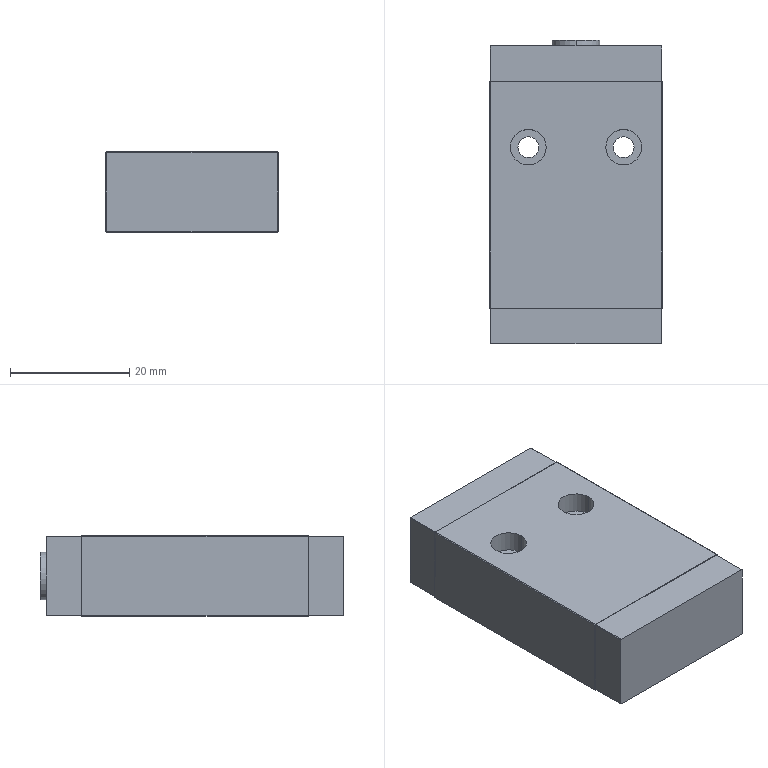Part | SolidWorks | features BaseBody 1 | 1 solid | 50 faces | box 29 x 51 x 13.5 mm | volume 18511 mm3 | plane 34 | cylinder 16 | commonest cylinder face diameters 6 x8 3.5 x4 5 x2 8 x2
STEP:
#1=CARTESIAN_POINT('',(-9.161,10.957,3.5));
#2=VERTEX_POINT('',#1);
#3=CARTESIAN_POINT('',(-15.161,10.957,3.5));
#4=VERTEX_POINT('',#3);
#5=CARTESIAN_POINT('',(-12.161,10.957,3.5));
#6=DIRECTION('',(0.,0.,-1.));
#7=DIRECTION('',(-1.,0.,0.));
#8=AXIS2_PLACEMENT_3D('',#5,#6,#7);
#9=CIRCLE('',#8,3.);
#10=EDGE_CURVE('',#2,#4,#9,.T.);
#11=ORIENTED_EDGE('',*,*,#10,.F.);
#12=CARTESIAN_POINT('',(-9.161,10.957,0.));
#13=VERTEX_POINT('',#12);
#14=CARTESIAN_POINT('',(-9.161,10.957,1.75));
#15=DIRECTION('',(0.,0.,-1.));
#16=VECTOR('',#15,1000.);
#17=LINE('',#14,#16);
#18=EDGE_CURVE('',#2,#13,#17,.T.);
#19=ORIENTED_EDGE('',*,*,#18,.T.);
#20=CARTESIAN_POINT('',(-15.161,10.957,0.));
#21=VERTEX_POINT('',#20);
#22=CARTESIAN_POINT('',(-12.161,10.957,0.));
#23=DIRECTION('',(0.,0.,-1.));
#24=DIRECTION('',(-1.,0.,0.));
#25=AXIS2_PLACEMENT_3D('',#22,#23,#24);
#26=CIRCLE('',#25,3.);
#27=EDGE_CURVE('',#13,#21,#26,.T.);
#28=ORIENTED_EDGE('',*,*,#27,.T.);
#29=CARTESIAN_POINT('',(-15.161,10.957,1.75));
#30=DIRECTION('',(0.,0.,-1.));
#31=VECTOR('',#30,1000.);
#32=LINE('',#29,#31);
#33=EDGE_CURVE('',#4,#21,#32,.T.);
#34=ORIENTED_EDGE('',*,*,#33,.F.);
#35=EDGE_LOOP('',(#11,#19,#28,#34));
#36=FACE_OUTER_BOUND('',#35,.T.);
#37=CARTESIAN_POINT('',(-12.161,10.957,1.75));
#38=DIRECTION('',(0.,0.,-1.));
#39=DIRECTION('',(-1.,0.,0.));
#40=AXIS2_PLACEMENT_3D('',#37,#38,#39);
#41=CYLINDRICAL_SURFACE('',#40,3.);
#42=ADVANCED_FACE('',(#36),#41,.F.);
#43=CARTESIAN_POINT('',(6.839,10.957,3.5));
#44=VERTEX_POINT('',#43);
#45=CARTESIAN_POINT('',(0.8387,10.957,3.5));
#46=VERTEX_POINT('',#45);
#47=CARTESIAN_POINT('',(3.839,10.957,3.5));
#48=DIRECTION('',(0.,0.,-1.));
#49=DIRECTION('',(-1.,0.,0.));
#50=AXIS2_PLACEMENT_3D('',#47,#48,#49);
#51=CIRCLE('',#50,3.);
#52=EDGE_CURVE('',#44,#46,#51,.T.);
#53=ORIENTED_EDGE('',*,*,#52,.F.);
#54=CARTESIAN_POINT('',(6.839,10.957,0.));
#55=VERTEX_POINT('',#54);
#56=CARTESIAN_POINT('',(6.839,10.957,1.75));
#57=DIRECTION('',(0.,0.,-1.));
#58=VECTOR('',#57,1000.);
#59=LINE('',#56,#58);
#60=EDGE_CURVE('',#44,#55,#59,.T.);
#61=ORIENTED_EDGE('',*,*,#60,.T.);
#62=CARTESIAN_POINT('',(0.8387,10.957,0.));
#63=VERTEX_POINT('',#62);
#64=CARTESIAN_POINT('',(3.839,10.957,0.));
#65=DIRECTION('',(0.,0.,-1.));
#66=DIRECTION('',(-1.,0.,0.));
#67=AXIS2_PLACEMENT_3D('',#64,#65,#66);
#68=CIRCLE('',#67,3.);
#69=EDGE_CURVE('',#55,#63,#68,.T.);
#70=ORIENTED_EDGE('',*,*,#69,.T.);
#71=CARTESIAN_POINT('',(0.8387,10.957,1.75));
#72=DIRECTION('',(0.,0.,-1.));
#73=VECTOR('',#72,1000.);
#74=LINE('',#71,#73);
#75=EDGE_CURVE('',#46,#63,#74,.T.);
#76=ORIENTED_EDGE('',*,*,#75,.F.);
#77=EDGE_LOOP('',(#53,#61,#70,#76));
#78=FACE_OUTER_BOUND('',#77,.T.);
#79=CARTESIAN_POINT('',(3.839,10.957,1.75));
#80=DIRECTION('',(0.,0.,-1.));
#81=DIRECTION('',(-1.,0.,0.));
#82=AXIS2_PLACEMENT_3D('',#79,#80,#81);
#83=CYLINDRICAL_SURFACE('',#82,3.);
#84=ADVANCED_FACE('',(#78),#83,.F.);
#85=CARTESIAN_POINT('',(-13.911,10.957,3.5));
#86=VERTEX_POINT('',#85);
#87=CARTESIAN_POINT('',(-10.411,10.957,3.5));
#88=VERTEX_POINT('',#87);
#89=CARTESIAN_POINT('',(-12.161,10.957,3.5));
#90=DIRECTION('',(0.,0.,1.));
#91=DIRECTION('',(1.,0.,0.));
#92=AXIS2_PLACEMENT_3D('',#89,#90,#91);
#93=CIRCLE('',#92,1.75);
#94=EDGE_CURVE('',#86,#88,#93,.T.);
#95=ORIENTED_EDGE('',*,*,#94,.F.);
#96=CARTESIAN_POINT('',(-13.911,10.957,10.));
#97=VERTEX_POINT('',#96);
#98=CARTESIAN_POINT('',(-13.911,10.957,-36.171));
#99=DIRECTION('',(0.,0.,1.));
#100=VECTOR('',#99,1000.);
#101=LINE('',#98,#100);
#102=EDGE_CURVE('',#86,#97,#101,.T.);
#103=ORIENTED_EDGE('',*,*,#102,.T.);
#104=CARTESIAN_POINT('',(-10.411,10.957,10.));
#105=VERTEX_POINT('',#104);
#106=CARTESIAN_POINT('',(-12.161,10.957,10.));
#107=DIRECTION('',(0.,0.,-1.));
#108=DIRECTION('',(1.,0.,0.));
#109=AXIS2_PLACEMENT_3D('',#106,#107,#108);
#110=CIRCLE('',#109,1.75);
#111=EDGE_CURVE('',#105,#97,#110,.T.);
#112=ORIENTED_EDGE('',*,*,#111,.F.);
#113=CARTESIAN_POINT('',(-10.411,10.957,-36.171));
#114=DIRECTION('',(0.,0.,1.));
#115=VECTOR('',#114,1000.);
#116=LINE('',#113,#115);
#117=EDGE_CURVE('',#88,#105,#116,.T.);
#118=ORIENTED_EDGE('',*,*,#117,.F.);
#119=EDGE_LOOP('',(#95,#103,#112,#118));
#120=FACE_OUTER_BOUND('',#119,.T.);
#121=CARTESIAN_POINT('',(-12.161,10.957,-36.171));
#122=DIRECTION('',(0.,0.,1.));
#123=DIRECTION('',(1.,0.,0.));
#124=AXIS2_PLACEMENT_3D('',#121,#122,#123);
#125=CYLINDRICAL_SURFACE('',#124,1.75);
#126=ADVANCED_FACE('',(#120),#125,.F.);
#127=CARTESIAN_POINT('',(2.089,10.957,3.5));
#128=VERTEX_POINT('',#127);
#129=CARTESIAN_POINT('',(5.589,10.957,3.5));
#130=VERTEX_POINT('',#129);
#131=CARTESIAN_POINT('',(3.839,10.957,3.5));
#132=DIRECTION('',(0.,0.,1.));
#133=DIRECTION('',(1.,0.,0.));
#134=AXIS2_PLACEMENT_3D('',#131,#132,#133);
#135=CIRCLE('',#134,1.75);
#136=EDGE_CURVE('',#128,#130,#135,.T.);
#137=ORIENTED_EDGE('',*,*,#136,.F.);
#138=CARTESIAN_POINT('',(2.089,10.957,10.));
#139=VERTEX_POINT('',#138);
#140=CARTESIAN_POINT('',(2.089,10.957,-36.171));
#141=DIRECTION('',(0.,0.,1.));
#142=VECTOR('',#141,1000.);
#143=LINE('',#140,#142);
#144=EDGE_CURVE('',#128,#139,#143,.T.);
#145=ORIENTED_EDGE('',*,*,#144,.T.);
#146=CARTESIAN_POINT('',(5.589,10.957,10.));
#147=VERTEX_POINT('',#146);
#148=CARTESIAN_POINT('',(3.839,10.957,10.));
#149=DIRECTION('',(0.,0.,-1.));
#150=DIRECTION('',(1.,0.,0.));
#151=AXIS2_PLACEMENT_3D('',#148,#149,#150);
#152=CIRCLE('',#151,1.75);
#153=EDGE_CURVE('',#147,#139,#152,.T.);
#154=ORIENTED_EDGE('',*,*,#153,.F.);
#155=CARTESIAN_POINT('',(5.589,10.957,-36.171));
#156=DIRECTION('',(0.,0.,1.));
#157=VECTOR('',#156,1000.);
#158=LINE('',#155,#157);
#159=EDGE_CURVE('',#130,#147,#158,.T.);
#160=ORIENTED_EDGE('',*,*,#159,.F.);
#161=EDGE_LOOP('',(#137,#145,#154,#160));
#162=FACE_OUTER_BOUND('',#161,.T.);
#163=CARTESIAN_POINT('',(3.839,10.957,-36.171));
#164=DIRECTION('',(0.,0.,1.));
#165=DIRECTION('',(1.,0.,0.));
#166=AXIS2_PLACEMENT_3D('',#163,#164,#165);
#167=CYLINDRICAL_SURFACE('',#166,1.75);
#168=ADVANCED_FACE('',(#162),#167,.F.);
#169=CARTESIAN_POINT('',(0.8387,10.957,10.));
#170=VERTEX_POINT('',#169);
#171=CARTESIAN_POINT('',(6.839,10.957,10.));
#172=VERTEX_POINT('',#171);
#173=CARTESIAN_POINT('',(3.839,10.957,10.));
#174=DIRECTION('',(0.,0.,1.));
#175=DIRECTION('',(1.,0.,0.));
#176=AXIS2_PLACEMENT_3D('',#173,#174,#175);
#177=CIRCLE('',#176,3.);
#178=EDGE_CURVE('',#170,#172,#177,.T.);
#179=ORIENTED_EDGE('',*,*,#178,.F.);
#180=CARTESIAN_POINT('',(0.8387,10.957,13.5));
#181=VERTEX_POINT('',#180);
#182=CARTESIAN_POINT('',(0.8387,10.957,11.75));
#183=DIRECTION('',(0.,0.,1.));
#184=VECTOR('',#183,1000.);
#185=LINE('',#182,#184);
#186=EDGE_CURVE('',#170,#181,#185,.T.);
#187=ORIENTED_EDGE('',*,*,#186,.T.);
#188=CARTESIAN_POINT('',(6.839,10.957,13.5));
#189=VERTEX_POINT('',#188);
#190=CARTESIAN_POINT('',(3.839,10.957,13.5));
#191=DIRECTION('',(0.,0.,-1.));
#192=DIRECTION('',(1.,0.,0.));
#193=AXIS2_PLACEMENT_3D('',#190,#191,#192);
#194=CIRCLE('',#193,3.);
#195=EDGE_CURVE('',#189,#181,#194,.T.);
#196=ORIENTED_EDGE('',*,*,#195,.F.);
#197=CARTESIAN_POINT('',(6.839,10.957,11.75));
#198=DIRECTION('',(0.,0.,1.));
#199=VECTOR('',#198,1000.);
#200=LINE('',#197,#199);
#201=EDGE_CURVE('',#172,#189,#200,.T.);
#202=ORIENTED_EDGE('',*,*,#201,.F.);
#203=EDGE_LOOP('',(#179,#187,#196,#202));
#204=FACE_OUTER_BOUND('',#203,.T.);
#205=CARTESIAN_POINT('',(3.839,10.957,11.75));
#206=DIRECTION('',(0.,0.,1.));
#207=DIRECTION('',(1.,0.,0.));
#208=AXIS2_PLACEMENT_3D('',#205,#206,#207);
#209=CYLINDRICAL_SURFACE('',#208,3.);
#210=ADVANCED_FACE('',(#204),#209,.F.);
#211=CARTESIAN_POINT('',(-15.161,10.957,10.));
#212=VERTEX_POINT('',#211);
#213=CARTESIAN_POINT('',(-9.161,10.957,10.));
#214=VERTEX_POINT('',#213);
#215=CARTESIAN_POINT('',(-12.161,10.957,10.));
#216=DIRECTION('',(0.,0.,1.));
#217=DIRECTION('',(1.,0.,0.));
#218=AXIS2_PLACEMENT_3D('',#215,#216,#217);
#219=CIRCLE('',#218,3.);
#220=EDGE_CURVE('',#212,#214,#219,.T.);
#221=ORIENTED_EDGE('',*,*,#220,.F.);
#222=CARTESIAN_POINT('',(-15.161,10.957,13.5));
#223=VERTEX_POINT('',#222);
#224=CARTESIAN_POINT('',(-15.161,10.957,11.75));
#225=DIRECTION('',(0.,0.,1.));
#226=VECTOR('',#225,1000.);
#227=LINE('',#224,#226);
#228=EDGE_CURVE('',#212,#223,#227,.T.);
#229=ORIENTED_EDGE('',*,*,#228,.T.);
#230=CARTESIAN_POINT('',(-9.161,10.957,13.5));
#231=VERTEX_POINT('',#230);
#232=CARTESIAN_POINT('',(-12.161,10.957,13.5));
#233=DIRECTION('',(0.,0.,-1.));
#234=DIRECTION('',(1.,0.,0.));
#235=AXIS2_PLACEMENT_3D('',#232,#233,#234);
#236=CIRCLE('',#235,3.);
#237=EDGE_CURVE('',#231,#223,#236,.T.);
#238=ORIENTED_EDGE('',*,*,#237,.F.);
#239=CARTESIAN_POINT('',(-9.161,10.957,11.75));
#240=DIRECTION('',(0.,0.,1.));
#241=VECTOR('',#240,1000.);
#242=LINE('',#239,#241);
#243=EDGE_CURVE('',#214,#231,#242,.T.);
#244=ORIENTED_EDGE('',*,*,#243,.F.);
#245=EDGE_LOOP('',(#221,#229,#238,#244));
#246=FACE_OUTER_BOUND('',#245,.T.);
#247=CARTESIAN_POINT('',(-12.161,10.957,11.75));
#248=DIRECTION('',(0.,0.,1.));
#249=DIRECTION('',(1.,0.,0.));
#250=AXIS2_PLACEMENT_3D('',#247,#248,#249);
#251=CYLINDRICAL_SURFACE('',#250,3.);
#252=ADVANCED_FACE('',(#246),#251,.F.);
#253=CARTESIAN_POINT('',(-4.161,27.957,2.75));
#254=VERTEX_POINT('',#253);
#255=CARTESIAN_POINT('',(-4.161,27.957,10.75));
#256=VERTEX_POINT('',#255);
#257=CARTESIAN_POINT('',(-4.161,27.957,6.75));
#258=DIRECTION('',(0.,-1.,0.));
#259=DIRECTION('',(0.,0.,1.));
#260=AXIS2_PLACEMENT_3D('',#257,#258,#259);
#261=CIRCLE('',#260,4.);
#262=EDGE_CURVE('',#254,#256,#261,.T.);
#263=ORIENTED_EDGE('',*,*,#262,.F.);
#264=CARTESIAN_POINT('',(-4.161,28.957,2.75));
#265=VERTEX_POINT('',#264);
#266=CARTESIAN_POINT('',(-4.161,27.957,2.75));
#267=DIRECTION('',(0.,1.,0.));
#268=VECTOR('',#267,1000.);
#269=LINE('',#266,#268);
#270=EDGE_CURVE('',#254,#265,#269,.T.);
#271=ORIENTED_EDGE('',*,*,#270,.T.);
#272=CARTESIAN_POINT('',(-4.161,28.957,10.75));
#273=VERTEX_POINT('',#272);
#274=CARTESIAN_POINT('',(-4.161,28.957,6.75));
#275=DIRECTION('',(0.,-1.,0.));
#276=DIRECTION('',(0.,0.,1.));
#277=AXIS2_PLACEMENT_3D('',#274,#275,#276);
#278=CIRCLE('',#277,4.);
#279=EDGE_CURVE('',#265,#273,#278,.T.);
#280=ORIENTED_EDGE('',*,*,#279,.T.);
#281=CARTESIAN_POINT('',(-4.161,27.957,10.75));
#282=DIRECTION('',(0.,1.,0.));
#283=VECTOR('',#282,1000.);
#284=LINE('',#281,#283);
#285=EDGE_CURVE('',#256,#273,#284,.T.);
#286=ORIENTED_EDGE('',*,*,#285,.F.);
#287=EDGE_LOOP('',(#263,#271,#280,#286));
#288=FACE_OUTER_BOUND('',#287,.T.);
#289=CARTESIAN_POINT('',(-4.161,27.957,6.75));
#290=DIRECTION('',(0.,1.,0.));
#291=DIRECTION('',(0.,0.,1.));
#292=AXIS2_PLACEMENT_3D('',#289,#290,#291);
#293=CYLINDRICAL_SURFACE('',#292,4.);
#294=ADVANCED_FACE('',(#288),#293,.T.);
#295=CARTESIAN_POINT('',(-1.661,3.957,6.75));
#296=VERTEX_POINT('',#295);
#297=CARTESIAN_POINT('',(-6.661,3.957,6.75));
#298=VERTEX_POINT('',#297);
#299=CARTESIAN_POINT('',(-4.161,3.957,6.75));
#300=DIRECTION('',(0.,1.,0.));
#301=DIRECTION('',(-1.,0.,0.));
#302=AXIS2_PLACEMENT_3D('',#299,#300,#301);
#303=CIRCLE('',#302,2.5);
#304=EDGE_CURVE('',#296,#298,#303,.T.);
#305=ORIENTED_EDGE('',*,*,#304,.F.);
#306=CARTESIAN_POINT('',(-1.661,28.957,6.75));
#307=VERTEX_POINT('',#306);
#308=CARTESIAN_POINT('',(-1.661,16.457,6.75));
#309=DIRECTION('',(0.,1.,0.));
#310=VECTOR('',#309,1000.);
#311=LINE('',#308,#310);
#312=EDGE_CURVE('',#296,#307,#311,.T.);
#313=ORIENTED_EDGE('',*,*,#312,.T.);
#314=CARTESIAN_POINT('',(-6.661,28.957,6.75));
#315=VERTEX_POINT('',#314);
#316=CARTESIAN_POINT('',(-4.161,28.957,6.75));
#317=DIRECTION('',(0.,1.,0.));
#318=DIRECTION('',(-1.,0.,0.));
#319=AXIS2_PLACEMENT_3D('',#316,#317,#318);
#320=CIRCLE('',#319,2.5);
#321=EDGE_CURVE('',#307,#315,#320,.T.);
#322=ORIENTED_EDGE('',*,*,#321,.T.);
#323=CARTESIAN_POINT('',(-6.661,16.457,6.75));
#324=DIRECTION('',(0.,1.,0.));
#325=VECTOR('',#324,1000.);
#326=LINE('',#323,#325);
#327=EDGE_CURVE('',#298,#315,#326,.T.);
#328=ORIENTED_EDGE('',*,*,#327,.F.);
#329=EDGE_LOOP('',(#305,#313,#322,#328));
#330=FACE_OUTER_BOUND('',#329,.T.);
#331=CARTESIAN_POINT('',(-4.161,16.457,6.75));
#332=DIRECTION('',(0.,1.,0.));
#333=DIRECTION('',(-1.,0.,0.));
#334=AXIS2_PLACEMENT_3D('',#331,#332,#333);
#335=CYLINDRICAL_SURFACE('',#334,2.5);
#336=ADVANCED_FACE('',(#330),#335,.F.);
#337=CARTESIAN_POINT('',(-12.161,10.957,0.));
#338=DIRECTION('',(0.,0.,-1.));
#339=DIRECTION('',(-1.,0.,0.));
#340=AXIS2_PLACEMENT_3D('',#337,#338,#339);
#341=CIRCLE('',#340,3.);
#342=EDGE_CURVE('',#21,#13,#341,.T.);
#343=ORIENTED_EDGE('',*,*,#342,.F.);
#344=ORIENTED_EDGE('',*,*,#27,.F.);
#345=EDGE_LOOP('',(#343,#344));
#346=FACE_BOUND('',#345,.T.);
#347=CARTESIAN_POINT('',(3.839,10.957,0.));
#348=DIRECTION('',(0.,0.,-1.));
#349=DIRECTION('',(-1.,0.,0.));
#350=AXIS2_PLACEMENT_3D('',#347,#348,#349);
#351=CIRCLE('',#350,3.);
#352=EDGE_CURVE('',#63,#55,#351,.T.);
#353=ORIENTED_EDGE('',*,*,#352,.F.);
#354=ORIENTED_EDGE('',*,*,#69,.F.);
#355=EDGE_LOOP('',(#353,#354));
#356=FACE_BOUND('',#355,.T.);
#357=CARTESIAN_POINT('',(10.239,21.957,0.));
#358=VERTEX_POINT('',#357);
#359=CARTESIAN_POINT('',(-18.561,21.957,0.));
#360=VERTEX_POINT('',#359);
#361=CARTESIAN_POINT('',(-4.161,21.957,0.));
#362=DIRECTION('',(-1.,0.,0.));
#363=VECTOR('',#362,1000.);
#364=LINE('',#361,#363);
#365=EDGE_CURVE('',#358,#360,#364,.T.);
#366=ORIENTED_EDGE('',*,*,#365,.F.);
#367=CARTESIAN_POINT('',(10.239,-16.043,0.));
#368=VERTEX_POINT('',#367);
#369=CARTESIAN_POINT('',(10.239,2.957,0.));
#370=DIRECTION('',(0.,1.,0.));
#371=VECTOR('',#370,1000.);
#372=LINE('',#369,#371);
#373=EDGE_CURVE('',#368,#358,#372,.T.);
#374=ORIENTED_EDGE('',*,*,#373,.F.);
#375=CARTESIAN_POINT('',(-18.561,-16.043,0.));
#376=VERTEX_POINT('',#375);
#377=CARTESIAN_POINT('',(-4.161,-16.043,0.));
#378=DIRECTION('',(1.,0.,0.));
#379=VECTOR('',#378,1000.);
#380=LINE('',#377,#379);
#381=EDGE_CURVE('',#376,#368,#380,.T.);
#382=ORIENTED_EDGE('',*,*,#381,.F.);
#383=CARTESIAN_POINT('',(-18.561,2.957,0.));
#384=DIRECTION('',(0.,-1.,0.));
#385=VECTOR('',#384,1000.);
#386=LINE('',#383,#385);
#387=EDGE_CURVE('',#360,#376,#386,.T.);
#388=ORIENTED_EDGE('',*,*,#387,.F.);
#389=EDGE_LOOP('',(#366,#374,#382,#388));
#390=FACE_OUTER_BOUND('',#389,.T.);
#391=CARTESIAN_POINT('',(-4.161,2.957,0.));
#392=DIRECTION('',(0.,0.,1.));
#393=DIRECTION('',(1.,0.,0.));
#394=AXIS2_PLACEMENT_3D('',#391,#392,#393);
#395=PLANE('',#394);
#396=ADVANCED_FACE('',(#346,#356,#390),#395,.F.);
#397=ORIENTED_EDGE('',*,*,#18,.F.);
#398=CARTESIAN_POINT('',(-12.161,10.957,3.5));
#399=DIRECTION('',(0.,0.,-1.));
#400=DIRECTION('',(-1.,0.,0.));
#401=AXIS2_PLACEMENT_3D('',#398,#399,#400);
#402=CIRCLE('',#401,3.);
#403=EDGE_CURVE('',#4,#2,#402,.T.);
#404=ORIENTED_EDGE('',*,*,#403,.F.);
#405=ORIENTED_EDGE('',*,*,#33,.T.);
#406=ORIENTED_EDGE('',*,*,#342,.T.);
#407=EDGE_LOOP('',(#397,#404,#405,#406));
#408=FACE_OUTER_BOUND('',#407,.T.);
#409=CARTESIAN_POINT('',(-12.161,10.957,1.75));
#410=DIRECTION('',(0.,0.,-1.));
#411=DIRECTION('',(-1.,0.,0.));
#412=AXIS2_PLACEMENT_3D('',#409,#410,#411);
#413=CYLINDRICAL_SURFACE('',#412,3.);
#414=ADVANCED_FACE('',(#408),#413,.F.);
#415=ORIENTED_EDGE('',*,*,#60,.F.);
#416=CARTESIAN_POINT('',(3.839,10.957,3.5));
#417=DIRECTION('',(0.,0.,-1.));
#418=DIRECTION('',(-1.,0.,0.));
#419=AXIS2_PLACEMENT_3D('',#416,#417,#418);
#420=CIRCLE('',#419,3.);
#421=EDGE_CURVE('',#46,#44,#420,.T.);
#422=ORIENTED_EDGE('',*,*,#421,.F.);
#423=ORIENTED_EDGE('',*,*,#75,.T.);
#424=ORIENTED_EDGE('',*,*,#352,.T.);
#425=EDGE_LOOP('',(#415,#422,#423,#424));
#426=FACE_OUTER_BOUND('',#425,.T.);
#427=CARTESIAN_POINT('',(3.839,10.957,1.75));
#428=DIRECTION('',(0.,0.,-1.));
#429=DIRECTION('',(-1.,0.,0.));
#430=AXIS2_PLACEMENT_3D('',#427,#428,#429);
#431=CYLINDRICAL_SURFACE('',#430,3.);
#432=ADVANCED_FACE('',(#426),#431,.F.);
#433=CARTESIAN_POINT('',(-18.661,-16.043,0.1));
#434=VERTEX_POINT('',#433);
#435=CARTESIAN_POINT('',(-18.611,-16.043,0.05));
#436=DIRECTION('',(-0.7071,0.,0.7071));
#437=VECTOR('',#436,1000.);
#438=LINE('',#435,#437);
#439=EDGE_CURVE('',#376,#434,#438,.T.);
#440=ORIENTED_EDGE('',*,*,#439,.T.);
#441=CARTESIAN_POINT('',(-18.661,21.957,0.1));
#442=VERTEX_POINT('',#441);
#443=CARTESIAN_POINT('',(-18.661,-6.543,0.1));
#444=DIRECTION('',(0.,1.,0.));
#445=VECTOR('',#444,1000.);
#446=LINE('',#443,#445);
#447=EDGE_CURVE('',#434,#442,#446,.T.);
#448=ORIENTED_EDGE('',*,*,#447,.T.);
#449=CARTESIAN_POINT('',(-18.611,21.957,0.05));
#450=DIRECTION('',(0.7071,0.,-0.7071));
#451=VECTOR('',#450,1000.);
#452=LINE('',#449,#451);
#453=EDGE_CURVE('',#442,#360,#452,.T.);
#454=ORIENTED_EDGE('',*,*,#453,.T.);
#455=ORIENTED_EDGE('',*,*,#387,.T.);
#456=EDGE_LOOP('',(#440,#448,#454,#455));
#457=FACE_OUTER_BOUND('',#456,.T.);
#458=CARTESIAN_POINT('',(-18.611,-6.543,0.05));
#459=DIRECTION('',(-0.7071,0.,-0.7071));
#460=DIRECTION('',(-0.7071,0.,0.7071));
#461=AXIS2_PLACEMENT_3D('',#458,#459,#460);
#462=PLANE('',#461);
#463=ADVANCED_FACE('',(#457),#462,.T.);
#464=CARTESIAN_POINT('',(-18.461,21.957,0.1));
#465=VERTEX_POINT('',#464);
#466=CARTESIAN_POINT('',(10.139,21.957,0.1));
#467=VERTEX_POINT('',#466);
#468=CARTESIAN_POINT('',(-18.661,21.957,0.1));
#469=DIRECTION('',(1.,0.,0.));
#470=VECTOR('',#469,1000.);
#471=LINE('',#468,#470);
#472=EDGE_CURVE('',#465,#467,#471,.T.);
#473=ORIENTED_EDGE('',*,*,#472,.T.);
#474=CARTESIAN_POINT('',(10.239,21.957,0.2));
#475=VERTEX_POINT('',#474);
#476=CARTESIAN_POINT('',(10.189,21.957,0.15));
#477=DIRECTION('',(-0.7071,0.,-0.7071));
#478=VECTOR('',#477,1000.);
#479=LINE('',#476,#478);
#480=EDGE_CURVE('',#475,#467,#479,.T.);
#481=ORIENTED_EDGE('',*,*,#480,.F.);
#482=CARTESIAN_POINT('',(10.239,21.957,13.3));
#483=VERTEX_POINT('',#482);
#484=CARTESIAN_POINT('',(10.239,21.957,0.));
#485=DIRECTION('',(0.,0.,1.));
#486=VECTOR('',#485,1000.);
#487=LINE('',#484,#486);
#488=EDGE_CURVE('',#475,#483,#487,.T.);
#489=ORIENTED_EDGE('',*,*,#488,.T.);
#490=CARTESIAN_POINT('',(10.139,21.957,13.4));
#491=VERTEX_POINT('',#490);
#492=CARTESIAN_POINT('',(10.189,21.957,13.35));
#493=DIRECTION('',(0.7071,0.,-0.7071));
#494=VECTOR('',#493,1000.);
#495=LINE('',#492,#494);
#496=EDGE_CURVE('',#491,#483,#495,.T.);
#497=ORIENTED_EDGE('',*,*,#496,.F.);
#498=CARTESIAN_POINT('',(-18.461,21.957,13.4));
#499=VERTEX_POINT('',#498);
#500=CARTESIAN_POINT('',(-18.661,21.957,13.4));
#501=DIRECTION('',(-1.,0.,0.));
#502=VECTOR('',#501,1000.);
#503=LINE('',#500,#502);
#504=EDGE_CURVE('',#491,#499,#503,.T.);
#505=ORIENTED_EDGE('',*,*,#504,.T.);
#506=CARTESIAN_POINT('',(-18.561,21.957,13.3));
#507=VERTEX_POINT('',#506);
#508=CARTESIAN_POINT('',(-18.511,21.957,13.35));
#509=DIRECTION('',(0.7071,0.,0.7071));
#510=VECTOR('',#509,1000.);
#511=LINE('',#508,#510);
#512=EDGE_CURVE('',#507,#499,#511,.T.);
#513=ORIENTED_EDGE('',*,*,#512,.F.);
#514=CARTESIAN_POINT('',(-18.561,21.957,0.2));
#515=VERTEX_POINT('',#514);
#516=CARTESIAN_POINT('',(-18.561,21.957,0.));
#517=DIRECTION('',(0.,0.,-1.));
#518=VECTOR('',#517,1000.);
#519=LINE('',#516,#518);
#520=EDGE_CURVE('',#507,#515,#519,.T.);
#521=ORIENTED_EDGE('',*,*,#520,.T.);
#522=CARTESIAN_POINT('',(-18.511,21.957,0.15));
#523=DIRECTION('',(-0.7071,0.,0.7071));
#524=VECTOR('',#523,1000.);
#525=LINE('',#522,#524);
#526=EDGE_CURVE('',#465,#515,#525,.T.);
#527=ORIENTED_EDGE('',*,*,#526,.F.);
#528=EDGE_LOOP('',(#473,#481,#489,#497,#505,#513,#521,#527));
#529=FACE_BOUND('',#528,.T.);
#530=CARTESIAN_POINT('',(10.339,21.957,0.1));
#531=VERTEX_POINT('',#530);
#532=CARTESIAN_POINT('',(10.339,21.957,0.1));
#533=DIRECTION('',(-0.7071,0.,-0.7071));
#534=VECTOR('',#533,1000.);
#535=LINE('',#532,#534);
#536=EDGE_CURVE('',#531,#358,#535,.T.);
#537=ORIENTED_EDGE('',*,*,#536,.T.);
#538=ORIENTED_EDGE('',*,*,#365,.T.);
#539=ORIENTED_EDGE('',*,*,#453,.F.);
#540=CARTESIAN_POINT('',(-18.661,21.957,13.4));
#541=VERTEX_POINT('',#540);
#542=CARTESIAN_POINT('',(-18.661,21.957,0.));
#543=DIRECTION('',(0.,0.,1.));
#544=VECTOR('',#543,1000.);
#545=LINE('',#542,#544);
#546=EDGE_CURVE('',#442,#541,#545,.T.);
#547=ORIENTED_EDGE('',*,*,#546,.T.);
#548=CARTESIAN_POINT('',(-18.561,21.957,13.5));
#549=VERTEX_POINT('',#548);
#550=CARTESIAN_POINT('',(-18.611,21.957,13.45));
#551=DIRECTION('',(-0.7071,0.,-0.7071));
#552=VECTOR('',#551,1000.);
#553=LINE('',#550,#552);
#554=EDGE_CURVE('',#549,#541,#553,.T.);
#555=ORIENTED_EDGE('',*,*,#554,.F.);
#556=CARTESIAN_POINT('',(10.239,21.957,13.5));
#557=VERTEX_POINT('',#556);
#558=CARTESIAN_POINT('',(-18.661,21.957,13.5));
#559=DIRECTION('',(1.,0.,0.));
#560=VECTOR('',#559,1000.);
#561=LINE('',#558,#560);
#562=EDGE_CURVE('',#549,#557,#561,.T.);
#563=ORIENTED_EDGE('',*,*,#562,.T.);
#564=CARTESIAN_POINT('',(10.339,21.957,13.4));
#565=VERTEX_POINT('',#564);
#566=CARTESIAN_POINT('',(10.289,21.957,13.45));
#567=DIRECTION('',(-0.7071,0.,0.7071));
#568=VECTOR('',#567,1000.);
#569=LINE('',#566,#568);
#570=EDGE_CURVE('',#565,#557,#569,.T.);
#571=ORIENTED_EDGE('',*,*,#570,.F.);
#572=CARTESIAN_POINT('',(10.339,21.957,0.));
#573=DIRECTION('',(0.,0.,-1.));
#574=VECTOR('',#573,1000.);
#575=LINE('',#572,#574);
#576=EDGE_CURVE('',#565,#531,#575,.T.);
#577=ORIENTED_EDGE('',*,*,#576,.T.);
#578=EDGE_LOOP('',(#537,#538,#539,#547,#555,#563,#571,#577));
#579=FACE_OUTER_BOUND('',#578,.T.);
#580=CARTESIAN_POINT('',(-18.661,21.957,0.));
#581=DIRECTION('',(0.,1.,0.));
#582=DIRECTION('',(0.,0.,1.));
#583=AXIS2_PLACEMENT_3D('',#580,#581,#582);
#584=PLANE('',#583);
#585=ADVANCED_FACE('',(#529,#579),#584,.T.);
#586=ORIENTED_EDGE('',*,*,#536,.F.);
#587=CARTESIAN_POINT('',(10.339,-16.043,0.1));
#588=VERTEX_POINT('',#587);
#589=CARTESIAN_POINT('',(10.339,12.457,0.1));
#590=DIRECTION('',(0.,-1.,0.));
#591=VECTOR('',#590,1000.);
#592=LINE('',#589,#591);
#593=EDGE_CURVE('',#531,#588,#592,.T.);
#594=ORIENTED_EDGE('',*,*,#593,.T.);
#595=CARTESIAN_POINT('',(10.289,-16.043,0.05));
#596=DIRECTION('',(-0.7071,0.,-0.7071));
#597=VECTOR('',#596,1000.);
#598=LINE('',#595,#597);
#599=EDGE_CURVE('',#588,#368,#598,.T.);
#600=ORIENTED_EDGE('',*,*,#599,.T.);
#601=ORIENTED_EDGE('',*,*,#373,.T.);
#602=EDGE_LOOP('',(#586,#594,#600,#601));
#603=FACE_OUTER_BOUND('',#602,.T.);
#604=CARTESIAN_POINT('',(10.289,12.457,0.05));
#605=DIRECTION('',(0.7071,0.,-0.7071));
#606=DIRECTION('',(-0.7071,0.,-0.7071));
#607=AXIS2_PLACEMENT_3D('',#604,#605,#606);
#608=PLANE('',#607);
#609=ADVANCED_FACE('',(#603),#608,.T.);
#610=CARTESIAN_POINT('',(-18.461,-16.043,13.4));
#611=VERTEX_POINT('',#610);
#612=CARTESIAN_POINT('',(10.139,-16.043,13.4));
#613=VERTEX_POINT('',#612);
#614=CARTESIAN_POINT('',(10.339,-16.043,13.4));
#615=DIRECTION('',(1.,0.,0.));
#616=VECTOR('',#615,1000.);
#617=LINE('',#614,#616);
#618=EDGE_CURVE('',#611,#613,#617,.T.);
#619=ORIENTED_EDGE('',*,*,#618,.T.);
#620=CARTESIAN_POINT('',(10.239,-16.043,13.3));
#621=VERTEX_POINT('',#620);
#622=CARTESIAN_POINT('',(10.189,-16.043,13.35));
#623=DIRECTION('',(-0.7071,0.,0.7071));
#624=VECTOR('',#623,1000.);
#625=LINE('',#622,#624);
#626=EDGE_CURVE('',#621,#613,#625,.T.);
#627=ORIENTED_EDGE('',*,*,#626,.F.);
#628=CARTESIAN_POINT('',(10.239,-16.043,0.2));
#629=VERTEX_POINT('',#628);
#630=CARTESIAN_POINT('',(10.239,-16.043,0.));
#631=DIRECTION('',(0.,0.,-1.));
#632=VECTOR('',#631,1000.);
#633=LINE('',#630,#632);
#634=EDGE_CURVE('',#621,#629,#633,.T.);
#635=ORIENTED_EDGE('',*,*,#634,.T.);
#636=CARTESIAN_POINT('',(10.139,-16.043,0.1));
#637=VERTEX_POINT('',#636);
#638=CARTESIAN_POINT('',(10.189,-16.043,0.15));
#639=DIRECTION('',(0.7071,0.,0.7071));
#640=VECTOR('',#639,1000.);
#641=LINE('',#638,#640);
#642=EDGE_CURVE('',#637,#629,#641,.T.);
#643=ORIENTED_EDGE('',*,*,#642,.F.);
#644=CARTESIAN_POINT('',(-18.461,-16.043,0.1));
#645=VERTEX_POINT('',#644);
#646=CARTESIAN_POINT('',(10.339,-16.043,0.1));
#647=DIRECTION('',(-1.,0.,0.));
#648=VECTOR('',#647,1000.);
#649=LINE('',#646,#648);
#650=EDGE_CURVE('',#637,#645,#649,.T.);
#651=ORIENTED_EDGE('',*,*,#650,.T.);
#652=CARTESIAN_POINT('',(-18.561,-16.043,0.2));
#653=VERTEX_POINT('',#652);
#654=CARTESIAN_POINT('',(-18.511,-16.043,0.15));
#655=DIRECTION('',(0.7071,0.,-0.7071));
#656=VECTOR('',#655,1000.);
#657=LINE('',#654,#656);
#658=EDGE_CURVE('',#653,#645,#657,.T.);
#659=ORIENTED_EDGE('',*,*,#658,.F.);
#660=CARTESIAN_POINT('',(-18.561,-16.043,13.3));
#661=VERTEX_POINT('',#660);
#662=CARTESIAN_POINT('',(-18.561,-16.043,0.));
#663=DIRECTION('',(0.,0.,1.));
#664=VECTOR('',#663,1000.);
#665=LINE('',#662,#664);
#666=EDGE_CURVE('',#653,#661,#665,.T.);
#667=ORIENTED_EDGE('',*,*,#666,.T.);
#668=CARTESIAN_POINT('',(-18.511,-16.043,13.35));
#669=DIRECTION('',(-0.7071,0.,-0.7071));
#670=VECTOR('',#669,1000.);
#671=LINE('',#668,#670);
#672=EDGE_CURVE('',#611,#661,#671,.T.);
#673=ORIENTED_EDGE('',*,*,#672,.F.);
#674=EDGE_LOOP('',(#619,#627,#635,#643,#651,#659,#667,#673));
#675=FACE_BOUND('',#674,.T.);
#676=CARTESIAN_POINT('',(-18.661,-16.043,13.4));
#677=VERTEX_POINT('',#676);
#678=CARTESIAN_POINT('',(-18.561,-16.043,13.5));
#679=VERTEX_POINT('',#678);
#680=CARTESIAN_POINT('',(-18.611,-16.043,13.45));
#681=DIRECTION('',(0.7071,0.,0.7071));
#682=VECTOR('',#681,1000.);
#683=LINE('',#680,#682);
#684=EDGE_CURVE('',#677,#679,#683,.T.);
#685=ORIENTED_EDGE('',*,*,#684,.F.);
#686=CARTESIAN_POINT('',(-18.661,-16.043,0.));
#687=DIRECTION('',(0.,0.,-1.));
#688=VECTOR('',#687,1000.);
#689=LINE('',#686,#688);
#690=EDGE_CURVE('',#677,#434,#689,.T.);
#691=ORIENTED_EDGE('',*,*,#690,.T.);
#692=ORIENTED_EDGE('',*,*,#439,.F.);
#693=ORIENTED_EDGE('',*,*,#381,.T.);
#694=ORIENTED_EDGE('',*,*,#599,.F.);
#695=CARTESIAN_POINT('',(10.339,-16.043,13.4));
#696=VERTEX_POINT('',#695);
#697=CARTESIAN_POINT('',(10.339,-16.043,0.));
#698=DIRECTION('',(0.,0.,1.));
#699=VECTOR('',#698,1000.);
#700=LINE('',#697,#699);
#701=EDGE_CURVE('',#588,#696,#700,.T.);
#702=ORIENTED_EDGE('',*,*,#701,.T.);
#703=CARTESIAN_POINT('',(10.239,-16.043,13.5));
#704=VERTEX_POINT('',#703);
#705=CARTESIAN_POINT('',(10.289,-16.043,13.45));
#706=DIRECTION('',(0.7071,0.,-0.7071));
#707=VECTOR('',#706,1000.);
#708=LINE('',#705,#707);
#709=EDGE_CURVE('',#704,#696,#708,.T.);
#710=ORIENTED_EDGE('',*,*,#709,.F.);
#711=CARTESIAN_POINT('',(10.339,-16.043,13.5));
#712=DIRECTION('',(-1.,0.,0.));
#713=VECTOR('',#712,1000.);
#714=LINE('',#711,#713);
#715=EDGE_CURVE('',#704,#679,#714,.T.);
#716=ORIENTED_EDGE('',*,*,#715,.T.);
#717=EDGE_LOOP('',(#685,#691,#692,#693,#694,#702,#710,#716));
#718=FACE_OUTER_BOUND('',#717,.T.);
#719=CARTESIAN_POINT('',(10.339,-16.043,0.));
#720=DIRECTION('',(0.,-1.,0.));
#721=DIRECTION('',(0.,0.,-1.));
#722=AXIS2_PLACEMENT_3D('',#719,#720,#721);
#723=PLANE('',#722);
#724=ADVANCED_FACE('',(#675,#718),#723,.T.);
#725=CARTESIAN_POINT('',(-12.161,10.957,3.5));
#726=DIRECTION('',(0.,0.,1.));
#727=DIRECTION('',(1.,0.,0.));
#728=AXIS2_PLACEMENT_3D('',#725,#726,#727);
#729=CIRCLE('',#728,1.75);
#730=EDGE_CURVE('',#88,#86,#729,.T.);
#731=ORIENTED_EDGE('',*,*,#730,.T.);
#732=ORIENTED_EDGE('',*,*,#94,.T.);
#733=EDGE_LOOP('',(#731,#732));
#734=FACE_BOUND('',#733,.T.);
#735=ORIENTED_EDGE('',*,*,#403,.T.);
#736=ORIENTED_EDGE('',*,*,#10,.T.);
#737=EDGE_LOOP('',(#735,#736));
#738=FACE_OUTER_BOUND('',#737,.T.);
#739=CARTESIAN_POINT('',(-12.161,10.957,3.5));
#740=DIRECTION('',(0.,0.,-1.));
#741=DIRECTION('',(-1.,0.,0.));
#742=AXIS2_PLACEMENT_3D('',#739,#740,#741);
#743=PLANE('',#742);
#744=ADVANCED_FACE('',(#734,#738),#743,.T.);
#745=CARTESIAN_POINT('',(3.839,10.957,3.5));
#746=DIRECTION('',(0.,0.,1.));
#747=DIRECTION('',(1.,0.,0.));
#748=AXIS2_PLACEMENT_3D('',#745,#746,#747);
#749=CIRCLE('',#748,1.75);
#750=EDGE_CURVE('',#130,#128,#749,.T.);
#751=ORIENTED_EDGE('',*,*,#750,.T.);
#752=ORIENTED_EDGE('',*,*,#136,.T.);
#753=EDGE_LOOP('',(#751,#752));
#754=FACE_BOUND('',#753,.T.);
#755=ORIENTED_EDGE('',*,*,#421,.T.);
#756=ORIENTED_EDGE('',*,*,#52,.T.);
#757=EDGE_LOOP('',(#755,#756));
#758=FACE_OUTER_BOUND('',#757,.T.);
#759=CARTESIAN_POINT('',(3.839,10.957,3.5));
#760=DIRECTION('',(0.,0.,-1.));
#761=DIRECTION('',(-1.,0.,0.));
#762=AXIS2_PLACEMENT_3D('',#759,#760,#761);
#763=PLANE('',#762);
#764=ADVANCED_FACE('',(#754,#758),#763,.T.);
#765=CARTESIAN_POINT('',(-18.661,-16.043,13.4));
#766=DIRECTION('',(0.,1.,0.));
#767=VECTOR('',#766,1000.);
#768=LINE('',#765,#767);
#769=EDGE_CURVE('',#677,#541,#768,.T.);
#770=ORIENTED_EDGE('',*,*,#769,.T.);
#771=ORIENTED_EDGE('',*,*,#546,.F.);
#772=ORIENTED_EDGE('',*,*,#447,.F.);
#773=ORIENTED_EDGE('',*,*,#690,.F.);
#774=EDGE_LOOP('',(#770,#771,#772,#773));
#775=FACE_OUTER_BOUND('',#774,.T.);
#776=CARTESIAN_POINT('',(-18.661,-16.043,0.));
#777=DIRECTION('',(-1.,0.,0.));
#778=DIRECTION('',(0.,0.,1.));
#779=AXIS2_PLACEMENT_3D('',#776,#777,#778);
#780=PLANE('',#779);
#781=ADVANCED_FACE('',(#775),#780,.T.);
#782=CARTESIAN_POINT('',(10.139,27.957,0.1));
#783=VERTEX_POINT('',#782);
#784=CARTESIAN_POINT('',(10.139,21.957,0.1));
#785=DIRECTION('',(0.,-1.,0.));
#786=VECTOR('',#785,1000.);
#787=LINE('',#784,#786);
#788=EDGE_CURVE('',#783,#467,#787,.T.);
#789=ORIENTED_EDGE('',*,*,#788,.T.);
#790=ORIENTED_EDGE('',*,*,#472,.F.);
#791=CARTESIAN_POINT('',(-18.461,27.957,0.1));
#792=VERTEX_POINT('',#791);
#793=CARTESIAN_POINT('',(-18.461,21.957,0.1));
#794=DIRECTION('',(0.,1.,0.));
#795=VECTOR('',#794,1000.);
#796=LINE('',#793,#795);
#797=EDGE_CURVE('',#465,#792,#796,.T.);
#798=ORIENTED_EDGE('',*,*,#797,.T.);
#799=CARTESIAN_POINT('',(-18.561,27.957,0.1));
#800=DIRECTION('',(1.,0.,0.));
#801=VECTOR('',#800,1000.);
#802=LINE('',#799,#801);
#803=EDGE_CURVE('',#792,#783,#802,.T.);
#804=ORIENTED_EDGE('',*,*,#803,.T.);
#805=EDGE_LOOP('',(#789,#790,#798,#804));
#806=FACE_OUTER_BOUND('',#805,.T.);
#807=CARTESIAN_POINT('',(-18.561,21.957,0.1));
#808=DIRECTION('',(0.,0.,-1.));
#809=DIRECTION('',(-1.,0.,0.));
#810=AXIS2_PLACEMENT_3D('',#807,#808,#809);
#811=PLANE('',#810);
#812=ADVANCED_FACE('',(#806),#811,.T.);
#813=CARTESIAN_POINT('',(-18.561,27.957,13.3));
#814=VERTEX_POINT('',#813);
#815=CARTESIAN_POINT('',(-18.561,21.957,13.3));
#816=DIRECTION('',(0.,1.,0.));
#817=VECTOR('',#816,1000.);
#818=LINE('',#815,#817);
#819=EDGE_CURVE('',#507,#814,#818,.T.);
#820=ORIENTED_EDGE('',*,*,#819,.T.);
#821=CARTESIAN_POINT('',(-18.561,27.957,0.2));
#822=VERTEX_POINT('',#821);
#823=CARTESIAN_POINT('',(-18.561,27.957,13.4));
#824=DIRECTION('',(0.,0.,-1.));
#825=VECTOR('',#824,1000.);
#826=LINE('',#823,#825);
#827=EDGE_CURVE('',#814,#822,#826,.T.);
#828=ORIENTED_EDGE('',*,*,#827,.T.);
#829=CARTESIAN_POINT('',(-18.561,21.957,0.2));
#830=DIRECTION('',(0.,-1.,0.));
#831=VECTOR('',#830,1000.);
#832=LINE('',#829,#831);
#833=EDGE_CURVE('',#822,#515,#832,.T.);
#834=ORIENTED_EDGE('',*,*,#833,.T.);
#835=ORIENTED_EDGE('',*,*,#520,.F.);
#836=EDGE_LOOP('',(#820,#828,#834,#835));
#837=FACE_OUTER_BOUND('',#836,.T.);
#838=CARTESIAN_POINT('',(-18.561,21.957,13.4));
#839=DIRECTION('',(-1.,0.,0.));
#840=DIRECTION('',(0.,0.,1.));
#841=AXIS2_PLACEMENT_3D('',#838,#839,#840);
#842=PLANE('',#841);
#843=ADVANCED_FACE('',(#837),#842,.T.);
#844=CARTESIAN_POINT('',(10.139,27.957,13.4));
#845=VERTEX_POINT('',#844);
#846=CARTESIAN_POINT('',(10.139,21.957,13.4));
#847=DIRECTION('',(0.,1.,0.));
#848=VECTOR('',#847,1000.);
#849=LINE('',#846,#848);
#850=EDGE_CURVE('',#491,#845,#849,.T.);
#851=ORIENTED_EDGE('',*,*,#850,.T.);
#852=CARTESIAN_POINT('',(-18.461,27.957,13.4));
#853=VERTEX_POINT('',#852);
#854=CARTESIAN_POINT('',(10.239,27.957,13.4));
#855=DIRECTION('',(-1.,0.,0.));
#856=VECTOR('',#855,1000.);
#857=LINE('',#854,#856);
#858=EDGE_CURVE('',#845,#853,#857,.T.);
#859=ORIENTED_EDGE('',*,*,#858,.T.);
#860=CARTESIAN_POINT('',(-18.461,21.957,13.4));
#861=DIRECTION('',(0.,-1.,0.));
#862=VECTOR('',#861,1000.);
#863=LINE('',#860,#862);
#864=EDGE_CURVE('',#853,#499,#863,.T.);
#865=ORIENTED_EDGE('',*,*,#864,.T.);
#866=ORIENTED_EDGE('',*,*,#504,.F.);
#867=EDGE_LOOP('',(#851,#859,#865,#866));
#868=FACE_OUTER_BOUND('',#867,.T.);
#869=CARTESIAN_POINT('',(10.239,21.957,13.4));
#870=DIRECTION('',(0.,0.,1.));
#871=DIRECTION('',(1.,0.,0.));
#872=AXIS2_PLACEMENT_3D('',#869,#870,#871);
#873=PLANE('',#872);
#874=ADVANCED_FACE('',(#868),#873,.T.);
#875=CARTESIAN_POINT('',(10.239,27.957,13.3));
#876=VERTEX_POINT('',#875);
#877=CARTESIAN_POINT('',(10.239,21.957,13.3));
#878=DIRECTION('',(0.,-1.,0.));
#879=VECTOR('',#878,1000.);
#880=LINE('',#877,#879);
#881=EDGE_CURVE('',#876,#483,#880,.T.);
#882=ORIENTED_EDGE('',*,*,#881,.T.);
#883=ORIENTED_EDGE('',*,*,#488,.F.);
#884=CARTESIAN_POINT('',(10.239,27.957,0.2));
#885=VERTEX_POINT('',#884);
#886=CARTESIAN_POINT('',(10.239,21.957,0.2));
#887=DIRECTION('',(0.,1.,0.));
#888=VECTOR('',#887,1000.);
#889=LINE('',#886,#888);
#890=EDGE_CURVE('',#475,#885,#889,.T.);
#891=ORIENTED_EDGE('',*,*,#890,.T.);
#892=CARTESIAN_POINT('',(10.239,27.957,0.1));
#893=DIRECTION('',(0.,0.,1.));
#894=VECTOR('',#893,1000.);
#895=LINE('',#892,#894);
#896=EDGE_CURVE('',#885,#876,#895,.T.);
#897=ORIENTED_EDGE('',*,*,#896,.T.);
#898=EDGE_LOOP('',(#882,#883,#891,#897));
#899=FACE_OUTER_BOUND('',#898,.T.);
#900=CARTESIAN_POINT('',(10.239,21.957,0.1));
#901=DIRECTION('',(1.,0.,0.));
#902=DIRECTION('',(0.,0.,-1.));
#903=AXIS2_PLACEMENT_3D('',#900,#901,#902);
#904=PLANE('',#903);
#905=ADVANCED_FACE('',(#899),#904,.T.);
#906=CARTESIAN_POINT('',(10.339,21.957,13.4));
#907=DIRECTION('',(0.,-1.,0.));
#908=VECTOR('',#907,1000.);
#909=LINE('',#906,#908);
#910=EDGE_CURVE('',#565,#696,#909,.T.);
#911=ORIENTED_EDGE('',*,*,#910,.T.);
#912=ORIENTED_EDGE('',*,*,#701,.F.);
#913=ORIENTED_EDGE('',*,*,#593,.F.);
#914=ORIENTED_EDGE('',*,*,#576,.F.);
#915=EDGE_LOOP('',(#911,#912,#913,#914));
#916=FACE_OUTER_BOUND('',#915,.T.);
#917=CARTESIAN_POINT('',(10.339,21.957,0.));
#918=DIRECTION('',(1.,0.,0.));
#919=DIRECTION('',(0.,0.,-1.));
#920=AXIS2_PLACEMENT_3D('',#917,#918,#919);
#921=PLANE('',#920);
#922=ADVANCED_FACE('',(#916),#921,.T.);
#923=ORIENTED_EDGE('',*,*,#195,.T.);
#924=CARTESIAN_POINT('',(3.839,10.957,13.5));
#925=DIRECTION('',(0.,0.,-1.));
#926=DIRECTION('',(1.,0.,0.));
#927=AXIS2_PLACEMENT_3D('',#924,#925,#926);
#928=CIRCLE('',#927,3.);
#929=EDGE_CURVE('',#181,#189,#928,.T.);
#930=ORIENTED_EDGE('',*,*,#929,.T.);
#931=EDGE_LOOP('',(#923,#930));
#932=FACE_BOUND('',#931,.T.);
#933=ORIENTED_EDGE('',*,*,#237,.T.);
#934=CARTESIAN_POINT('',(-12.161,10.957,13.5));
#935=DIRECTION('',(0.,0.,-1.));
#936=DIRECTION('',(1.,0.,0.));
#937=AXIS2_PLACEMENT_3D('',#934,#935,#936);
#938=CIRCLE('',#937,3.);
#939=EDGE_CURVE('',#223,#231,#938,.T.);
#940=ORIENTED_EDGE('',*,*,#939,.T.);
#941=EDGE_LOOP('',(#933,#940));
#942=FACE_BOUND('',#941,.T.);
#943=CARTESIAN_POINT('',(10.239,2.957,13.5));
#944=DIRECTION('',(0.,1.,0.));
#945=VECTOR('',#944,1000.);
#946=LINE('',#943,#945);
#947=EDGE_CURVE('',#704,#557,#946,.T.);
#948=ORIENTED_EDGE('',*,*,#947,.T.);
#949=ORIENTED_EDGE('',*,*,#562,.F.);
#950=CARTESIAN_POINT('',(-18.561,2.957,13.5));
#951=DIRECTION('',(0.,-1.,0.));
#952=VECTOR('',#951,1000.);
#953=LINE('',#950,#952);
#954=EDGE_CURVE('',#549,#679,#953,.T.);
#955=ORIENTED_EDGE('',*,*,#954,.T.);
#956=ORIENTED_EDGE('',*,*,#715,.F.);
#957=EDGE_LOOP('',(#948,#949,#955,#956));
#958=FACE_OUTER_BOUND('',#957,.T.);
#959=CARTESIAN_POINT('',(-4.161,2.957,13.5));
#960=DIRECTION('',(0.,0.,1.));
#961=DIRECTION('',(1.,0.,0.));
#962=AXIS2_PLACEMENT_3D('',#959,#960,#961);
#963=PLANE('',#962);
#964=ADVANCED_FACE('',(#932,#942,#958),#963,.T.);
#965=CARTESIAN_POINT('',(10.139,-22.043,13.4));
#966=VERTEX_POINT('',#965);
#967=CARTESIAN_POINT('',(10.139,-16.043,13.4));
#968=DIRECTION('',(0.,1.,0.));
#969=VECTOR('',#968,1000.);
#970=LINE('',#967,#969);
#971=EDGE_CURVE('',#966,#613,#970,.T.);
#972=ORIENTED_EDGE('',*,*,#971,.T.);
#973=ORIENTED_EDGE('',*,*,#618,.F.);
#974=CARTESIAN_POINT('',(-18.461,-22.043,13.4));
#975=VERTEX_POINT('',#974);
#976=CARTESIAN_POINT('',(-18.461,-16.043,13.4));
#977=DIRECTION('',(0.,-1.,0.));
#978=VECTOR('',#977,1000.);
#979=LINE('',#976,#978);
#980=EDGE_CURVE('',#611,#975,#979,.T.);
#981=ORIENTED_EDGE('',*,*,#980,.T.);
#982=CARTESIAN_POINT('',(-18.561,-22.043,13.4));
#983=DIRECTION('',(1.,0.,0.));
#984=VECTOR('',#983,1000.);
#985=LINE('',#982,#984);
#986=EDGE_CURVE('',#975,#966,#985,.T.);
#987=ORIENTED_EDGE('',*,*,#986,.T.);
#988=EDGE_LOOP('',(#972,#973,#981,#987));
#989=FACE_OUTER_BOUND('',#988,.T.);
#990=CARTESIAN_POINT('',(-18.561,-16.043,13.4));
#991=DIRECTION('',(0.,0.,1.));
#992=DIRECTION('',(1.,0.,0.));
#993=AXIS2_PLACEMENT_3D('',#990,#991,#992);
#994=PLANE('',#993);
#995=ADVANCED_FACE('',(#989),#994,.T.);
#996=CARTESIAN_POINT('',(-18.561,-22.043,13.3));
#997=VERTEX_POINT('',#996);
#998=CARTESIAN_POINT('',(-18.561,-16.043,13.3));
#999=DIRECTION('',(0.,1.,0.));
#1000=VECTOR('',#999,1000.);
#1001=LINE('',#998,#1000);
#1002=EDGE_CURVE('',#997,#661,#1001,.T.);
#1003=ORIENTED_EDGE('',*,*,#1002,.T.);
#1004=ORIENTED_EDGE('',*,*,#666,.F.);
#1005=CARTESIAN_POINT('',(-18.561,-22.043,0.2));
#1006=VERTEX_POINT('',#1005);
#1007=CARTESIAN_POINT('',(-18.561,-16.043,0.2));
#1008=DIRECTION('',(0.,-1.,0.));
#1009=VECTOR('',#1008,1000.);
#1010=LINE('',#1007,#1009);
#1011=EDGE_CURVE('',#653,#1006,#1010,.T.);
#1012=ORIENTED_EDGE('',*,*,#1011,.T.);
#1013=CARTESIAN_POINT('',(-18.561,-22.043,0.1));
#1014=DIRECTION('',(0.,0.,1.));
#1015=VECTOR('',#1014,1000.);
#1016=LINE('',#1013,#1015);
#1017=EDGE_CURVE('',#1006,#997,#1016,.T.);
#1018=ORIENTED_EDGE('',*,*,#1017,.T.);
#1019=EDGE_LOOP('',(#1003,#1004,#1012,#1018));
#1020=FACE_OUTER_BOUND('',#1019,.T.);
#1021=CARTESIAN_POINT('',(-18.561,-16.043,0.1));
#1022=DIRECTION('',(-1.,0.,0.));
#1023=DIRECTION('',(0.,0.,1.));
#1024=AXIS2_PLACEMENT_3D('',#1021,#1022,#1023);
#1025=PLANE('',#1024);
#1026=ADVANCED_FACE('',(#1020),#1025,.T.);
#1027=CARTESIAN_POINT('',(10.139,-22.043,0.1));
#1028=VERTEX_POINT('',#1027);
#1029=CARTESIAN_POINT('',(10.139,-16.043,0.1));
#1030=DIRECTION('',(0.,-1.,0.));
#1031=VECTOR('',#1030,1000.);
#1032=LINE('',#1029,#1031);
#1033=EDGE_CURVE('',#637,#1028,#1032,.T.);
#1034=ORIENTED_EDGE('',*,*,#1033,.T.);
#1035=CARTESIAN_POINT('',(-18.461,-22.043,0.1));
#1036=VERTEX_POINT('',#1035);
#1037=CARTESIAN_POINT('',(10.239,-22.043,0.1));
#1038=DIRECTION('',(-1.,0.,0.));
#1039=VECTOR('',#1038,1000.);
#1040=LINE('',#1037,#1039);
#1041=EDGE_CURVE('',#1028,#1036,#1040,.T.);
#1042=ORIENTED_EDGE('',*,*,#1041,.T.);
#1043=CARTESIAN_POINT('',(-18.461,-16.043,0.1));
#1044=DIRECTION('',(0.,1.,0.));
#1045=VECTOR('',#1044,1000.);
#1046=LINE('',#1043,#1045);
#1047=EDGE_CURVE('',#1036,#645,#1046,.T.);
#1048=ORIENTED_EDGE('',*,*,#1047,.T.);
#1049=ORIENTED_EDGE('',*,*,#650,.F.);
#1050=EDGE_LOOP('',(#1034,#1042,#1048,#1049));
#1051=FACE_OUTER_BOUND('',#1050,.T.);
#1052=CARTESIAN_POINT('',(10.239,-16.043,0.1));
#1053=DIRECTION('',(0.,0.,-1.));
#1054=DIRECTION('',(-1.,0.,0.));
#1055=AXIS2_PLACEMENT_3D('',#1052,#1053,#1054);
#1056=PLANE('',#1055);
#1057=ADVANCED_FACE('',(#1051),#1056,.T.);
#1058=CARTESIAN_POINT('',(10.239,-22.043,13.3));
#1059=VERTEX_POINT('',#1058);
#1060=CARTESIAN_POINT('',(10.239,-16.043,13.3));
#1061=DIRECTION('',(0.,-1.,0.));
#1062=VECTOR('',#1061,1000.);
#1063=LINE('',#1060,#1062);
#1064=EDGE_CURVE('',#621,#1059,#1063,.T.);
#1065=ORIENTED_EDGE('',*,*,#1064,.T.);
#1066=CARTESIAN_POINT('',(10.239,-22.043,0.2));
#1067=VERTEX_POINT('',#1066);
#1068=CARTESIAN_POINT('',(10.239,-22.043,13.4));
#1069=DIRECTION('',(0.,0.,-1.));
#1070=VECTOR('',#1069,1000.);
#1071=LINE('',#1068,#1070);
#1072=EDGE_CURVE('',#1059,#1067,#1071,.T.);
#1073=ORIENTED_EDGE('',*,*,#1072,.T.);
#1074=CARTESIAN_POINT('',(10.239,-16.043,0.2));
#1075=DIRECTION('',(0.,1.,0.));
#1076=VECTOR('',#1075,1000.);
#1077=LINE('',#1074,#1076);
#1078=EDGE_CURVE('',#1067,#629,#1077,.T.);
#1079=ORIENTED_EDGE('',*,*,#1078,.T.);
#1080=ORIENTED_EDGE('',*,*,#634,.F.);
#1081=EDGE_LOOP('',(#1065,#1073,#1079,#1080));
#1082=FACE_OUTER_BOUND('',#1081,.T.);
#1083=CARTESIAN_POINT('',(10.239,-16.043,13.4));
#1084=DIRECTION('',(1.,0.,0.));
#1085=DIRECTION('',(0.,0.,-1.));
#1086=AXIS2_PLACEMENT_3D('',#1083,#1084,#1085);
#1087=PLANE('',#1086);
#1088=ADVANCED_FACE('',(#1082),#1087,.T.);
#1089=ORIENTED_EDGE('',*,*,#102,.F.);
#1090=ORIENTED_EDGE('',*,*,#730,.F.);
#1091=ORIENTED_EDGE('',*,*,#117,.T.);
#1092=CARTESIAN_POINT('',(-12.161,10.957,10.));
#1093=DIRECTION('',(0.,0.,-1.));
#1094=DIRECTION('',(1.,0.,0.));
#1095=AXIS2_PLACEMENT_3D('',#1092,#1093,#1094);
#1096=CIRCLE('',#1095,1.75);
#1097=EDGE_CURVE('',#97,#105,#1096,.T.);
#1098=ORIENTED_EDGE('',*,*,#1097,.F.);
#1099=EDGE_LOOP('',(#1089,#1090,#1091,#1098));
#1100=FACE_OUTER_BOUND('',#1099,.T.);
#1101=CARTESIAN_POINT('',(-12.161,10.957,-36.171));
#1102=DIRECTION('',(0.,0.,1.));
#1103=DIRECTION('',(1.,0.,0.));
#1104=AXIS2_PLACEMENT_3D('',#1101,#1102,#1103);
#1105=CYLINDRICAL_SURFACE('',#1104,1.75);
#1106=ADVANCED_FACE('',(#1100),#1105,.F.);
#1107=ORIENTED_EDGE('',*,*,#144,.F.);
#1108=ORIENTED_EDGE('',*,*,#750,.F.);
#1109=ORIENTED_EDGE('',*,*,#159,.T.);
#1110=CARTESIAN_POINT('',(3.839,10.957,10.));
#1111=DIRECTION('',(0.,0.,-1.));
#1112=DIRECTION('',(1.,0.,0.));
#1113=AXIS2_PLACEMENT_3D('',#1110,#1111,#1112);
#1114=CIRCLE('',#1113,1.75);
#1115=EDGE_CURVE('',#139,#147,#1114,.T.);
#1116=ORIENTED_EDGE('',*,*,#1115,.F.);
#1117=EDGE_LOOP('',(#1107,#1108,#1109,#1116));
#1118=FACE_OUTER_BOUND('',#1117,.T.);
#1119=CARTESIAN_POINT('',(3.839,10.957,-36.171));
#1120=DIRECTION('',(0.,0.,1.));
#1121=DIRECTION('',(1.,0.,0.));
#1122=AXIS2_PLACEMENT_3D('',#1119,#1120,#1121);
#1123=CYLINDRICAL_SURFACE('',#1122,1.75);
#1124=ADVANCED_FACE('',(#1118),#1123,.F.);
#1125=ORIENTED_EDGE('',*,*,#684,.T.);
#1126=ORIENTED_EDGE('',*,*,#954,.F.);
#1127=ORIENTED_EDGE('',*,*,#554,.T.);
#1128=ORIENTED_EDGE('',*,*,#769,.F.);
#1129=EDGE_LOOP('',(#1125,#1126,#1127,#1128));
#1130=FACE_OUTER_BOUND('',#1129,.T.);
#1131=CARTESIAN_POINT('',(-18.611,-6.543,13.45));
#1132=DIRECTION('',(-0.7071,0.,0.7071));
#1133=DIRECTION('',(0.7071,0.,0.7071));
#1134=AXIS2_PLACEMENT_3D('',#1131,#1132,#1133);
#1135=PLANE('',#1134);
#1136=ADVANCED_FACE('',(#1130),#1135,.T.);
#1137=ORIENTED_EDGE('',*,*,#480,.T.);
#1138=ORIENTED_EDGE('',*,*,#788,.F.);
#1139=CARTESIAN_POINT('',(10.189,27.957,0.15));
#1140=DIRECTION('',(0.7071,0.,0.7071));
#1141=VECTOR('',#1140,1000.);
#1142=LINE('',#1139,#1141);
#1143=EDGE_CURVE('',#783,#885,#1142,.T.);
#1144=ORIENTED_EDGE('',*,*,#1143,.T.);
#1145=ORIENTED_EDGE('',*,*,#890,.F.);
#1146=EDGE_LOOP('',(#1137,#1138,#1144,#1145));
#1147=FACE_OUTER_BOUND('',#1146,.T.);
#1148=CARTESIAN_POINT('',(10.189,21.957,0.15));
#1149=DIRECTION('',(0.7071,0.,-0.7071));
#1150=DIRECTION('',(-0.7071,0.,-0.7071));
#1151=AXIS2_PLACEMENT_3D('',#1148,#1149,#1150);
#1152=PLANE('',#1151);
#1153=ADVANCED_FACE('',(#1147),#1152,.T.);
#1154=CARTESIAN_POINT('',(-4.161,27.957,6.75));
#1155=DIRECTION('',(0.,-1.,0.));
#1156=DIRECTION('',(0.,0.,1.));
#1157=AXIS2_PLACEMENT_3D('',#1154,#1155,#1156);
#1158=CIRCLE('',#1157,4.);
#1159=EDGE_CURVE('',#256,#254,#1158,.T.);
#1160=ORIENTED_EDGE('',*,*,#1159,.T.);
#1161=ORIENTED_EDGE('',*,*,#262,.T.);
#1162=EDGE_LOOP('',(#1160,#1161));
#1163=FACE_BOUND('',#1162,.T.);
#1164=ORIENTED_EDGE('',*,*,#1143,.F.);
#1165=ORIENTED_EDGE('',*,*,#803,.F.);
#1166=CARTESIAN_POINT('',(-18.461,27.957,0.1));
#1167=DIRECTION('',(-0.7071,0.,0.7071));
#1168=VECTOR('',#1167,1000.);
#1169=LINE('',#1166,#1168);
#1170=EDGE_CURVE('',#792,#822,#1169,.T.);
#1171=ORIENTED_EDGE('',*,*,#1170,.T.);
#1172=ORIENTED_EDGE('',*,*,#827,.F.);
#1173=CARTESIAN_POINT('',(-18.561,27.957,13.3));
#1174=DIRECTION('',(0.7071,0.,0.7071));
#1175=VECTOR('',#1174,1000.);
#1176=LINE('',#1173,#1175);
#1177=EDGE_CURVE('',#814,#853,#1176,.T.);
#1178=ORIENTED_EDGE('',*,*,#1177,.T.);
#1179=ORIENTED_EDGE('',*,*,#858,.F.);
#1180=CARTESIAN_POINT('',(10.139,27.957,13.4));
#1181=DIRECTION('',(0.7071,0.,-0.7071));
#1182=VECTOR('',#1181,1000.);
#1183=LINE('',#1180,#1182);
#1184=EDGE_CURVE('',#845,#876,#1183,.T.);
#1185=ORIENTED_EDGE('',*,*,#1184,.T.);
#1186=ORIENTED_EDGE('',*,*,#896,.F.);
#1187=EDGE_LOOP('',(#1164,#1165,#1171,#1172,#1178,#1179,#1185,#1186));
#1188=FACE_OUTER_BOUND('',#1187,.T.);
#1189=CARTESIAN_POINT('',(-4.161,27.957,6.75));
#1190=DIRECTION('',(0.,1.,0.));
#1191=DIRECTION('',(0.,0.,1.));
#1192=AXIS2_PLACEMENT_3D('',#1189,#1190,#1191);
#1193=PLANE('',#1192);
#1194=ADVANCED_FACE('',(#1163,#1188),#1193,.T.);
#1195=ORIENTED_EDGE('',*,*,#526,.T.);
#1196=ORIENTED_EDGE('',*,*,#833,.F.);
#1197=ORIENTED_EDGE('',*,*,#1170,.F.);
#1198=ORIENTED_EDGE('',*,*,#797,.F.);
#1199=EDGE_LOOP('',(#1195,#1196,#1197,#1198));
#1200=FACE_OUTER_BOUND('',#1199,.T.);
#1201=CARTESIAN_POINT('',(-18.511,21.957,0.15));
#1202=DIRECTION('',(-0.7071,0.,-0.7071));
#1203=DIRECTION('',(-0.7071,0.,0.7071));
#1204=AXIS2_PLACEMENT_3D('',#1201,#1202,#1203);
#1205=PLANE('',#1204);
#1206=ADVANCED_FACE('',(#1200),#1205,.T.);
#1207=ORIENTED_EDGE('',*,*,#512,.T.);
#1208=ORIENTED_EDGE('',*,*,#864,.F.);
#1209=ORIENTED_EDGE('',*,*,#1177,.F.);
#1210=ORIENTED_EDGE('',*,*,#819,.F.);
#1211=EDGE_LOOP('',(#1207,#1208,#1209,#1210));
#1212=FACE_OUTER_BOUND('',#1211,.T.);
#1213=CARTESIAN_POINT('',(-18.511,21.957,13.35));
#1214=DIRECTION('',(-0.7071,0.,0.7071));
#1215=DIRECTION('',(0.7071,0.,0.7071));
#1216=AXIS2_PLACEMENT_3D('',#1213,#1214,#1215);
#1217=PLANE('',#1216);
#1218=ADVANCED_FACE('',(#1212),#1217,.T.);
#1219=ORIENTED_EDGE('',*,*,#496,.T.);
#1220=ORIENTED_EDGE('',*,*,#881,.F.);
#1221=ORIENTED_EDGE('',*,*,#1184,.F.);
#1222=ORIENTED_EDGE('',*,*,#850,.F.);
#1223=EDGE_LOOP('',(#1219,#1220,#1221,#1222));
#1224=FACE_OUTER_BOUND('',#1223,.T.);
#1225=CARTESIAN_POINT('',(10.189,21.957,13.35));
#1226=DIRECTION('',(0.7071,0.,0.7071));
#1227=DIRECTION('',(0.7071,0.,-0.7071));
#1228=AXIS2_PLACEMENT_3D('',#1225,#1226,#1227);
#1229=PLANE('',#1228);
#1230=ADVANCED_FACE('',(#1224),#1229,.T.);
#1231=ORIENTED_EDGE('',*,*,#570,.T.);
#1232=ORIENTED_EDGE('',*,*,#947,.F.);
#1233=ORIENTED_EDGE('',*,*,#709,.T.);
#1234=ORIENTED_EDGE('',*,*,#910,.F.);
#1235=EDGE_LOOP('',(#1231,#1232,#1233,#1234));
#1236=FACE_OUTER_BOUND('',#1235,.T.);
#1237=CARTESIAN_POINT('',(10.289,12.457,13.45));
#1238=DIRECTION('',(0.7071,0.,0.7071));
#1239=DIRECTION('',(0.7071,0.,-0.7071));
#1240=AXIS2_PLACEMENT_3D('',#1237,#1238,#1239);
#1241=PLANE('',#1240);
#1242=ADVANCED_FACE('',(#1236),#1241,.T.);
#1243=ORIENTED_EDGE('',*,*,#186,.F.);
#1244=CARTESIAN_POINT('',(3.839,10.957,10.));
#1245=DIRECTION('',(0.,0.,1.));
#1246=DIRECTION('',(1.,0.,0.));
#1247=AXIS2_PLACEMENT_3D('',#1244,#1245,#1246);
#1248=CIRCLE('',#1247,3.);
#1249=EDGE_CURVE('',#172,#170,#1248,.T.);
#1250=ORIENTED_EDGE('',*,*,#1249,.F.);
#1251=ORIENTED_EDGE('',*,*,#201,.T.);
#1252=ORIENTED_EDGE('',*,*,#929,.F.);
#1253=EDGE_LOOP('',(#1243,#1250,#1251,#1252));
#1254=FACE_OUTER_BOUND('',#1253,.T.);
#1255=CARTESIAN_POINT('',(3.839,10.957,11.75));
#1256=DIRECTION('',(0.,0.,1.));
#1257=DIRECTION('',(1.,0.,0.));
#1258=AXIS2_PLACEMENT_3D('',#1255,#1256,#1257);
#1259=CYLINDRICAL_SURFACE('',#1258,3.);
#1260=ADVANCED_FACE('',(#1254),#1259,.F.);
#1261=ORIENTED_EDGE('',*,*,#228,.F.);
#1262=CARTESIAN_POINT('',(-12.161,10.957,10.));
#1263=DIRECTION('',(0.,0.,1.));
#1264=DIRECTION('',(1.,0.,0.));
#1265=AXIS2_PLACEMENT_3D('',#1262,#1263,#1264);
#1266=CIRCLE('',#1265,3.);
#1267=EDGE_CURVE('',#214,#212,#1266,.T.);
#1268=ORIENTED_EDGE('',*,*,#1267,.F.);
#1269=ORIENTED_EDGE('',*,*,#243,.T.);
#1270=ORIENTED_EDGE('',*,*,#939,.F.);
#1271=EDGE_LOOP('',(#1261,#1268,#1269,#1270));
#1272=FACE_OUTER_BOUND('',#1271,.T.);
#1273=CARTESIAN_POINT('',(-12.161,10.957,11.75));
#1274=DIRECTION('',(0.,0.,1.));
#1275=DIRECTION('',(1.,0.,0.));
#1276=AXIS2_PLACEMENT_3D('',#1273,#1274,#1275);
#1277=CYLINDRICAL_SURFACE('',#1276,3.);
#1278=ADVANCED_FACE('',(#1272),#1277,.F.);
#1279=ORIENTED_EDGE('',*,*,#626,.T.);
#1280=ORIENTED_EDGE('',*,*,#971,.F.);
#1281=CARTESIAN_POINT('',(10.189,-22.043,13.35));
#1282=DIRECTION('',(0.7071,0.,-0.7071));
#1283=VECTOR('',#1282,1000.);
#1284=LINE('',#1281,#1283);
#1285=EDGE_CURVE('',#966,#1059,#1284,.T.);
#1286=ORIENTED_EDGE('',*,*,#1285,.T.);
#1287=ORIENTED_EDGE('',*,*,#1064,.F.);
#1288=EDGE_LOOP('',(#1279,#1280,#1286,#1287));
#1289=FACE_OUTER_BOUND('',#1288,.T.);
#1290=CARTESIAN_POINT('',(10.189,-16.043,13.35));
#1291=DIRECTION('',(0.7071,0.,0.7071));
#1292=DIRECTION('',(0.7071,0.,-0.7071));
#1293=AXIS2_PLACEMENT_3D('',#1290,#1291,#1292);
#1294=PLANE('',#1293);
#1295=ADVANCED_FACE('',(#1289),#1294,.T.);
#1296=ORIENTED_EDGE('',*,*,#1041,.F.);
#1297=CARTESIAN_POINT('',(10.239,-22.043,0.2));
#1298=DIRECTION('',(-0.7071,0.,-0.7071));
#1299=VECTOR('',#1298,1000.);
#1300=LINE('',#1297,#1299);
#1301=EDGE_CURVE('',#1067,#1028,#1300,.T.);
#1302=ORIENTED_EDGE('',*,*,#1301,.F.);
#1303=ORIENTED_EDGE('',*,*,#1072,.F.);
#1304=ORIENTED_EDGE('',*,*,#1285,.F.);
#1305=ORIENTED_EDGE('',*,*,#986,.F.);
#1306=CARTESIAN_POINT('',(-18.561,-22.043,13.3));
#1307=DIRECTION('',(0.7071,0.,0.7071));
#1308=VECTOR('',#1307,1000.);
#1309=LINE('',#1306,#1308);
#1310=EDGE_CURVE('',#997,#975,#1309,.T.);
#1311=ORIENTED_EDGE('',*,*,#1310,.F.);
#1312=ORIENTED_EDGE('',*,*,#1017,.F.);
#1313=CARTESIAN_POINT('',(-18.461,-22.043,0.1));
#1314=DIRECTION('',(-0.7071,0.,0.7071));
#1315=VECTOR('',#1314,1000.);
#1316=LINE('',#1313,#1315);
#1317=EDGE_CURVE('',#1036,#1006,#1316,.T.);
#1318=ORIENTED_EDGE('',*,*,#1317,.F.);
#1319=EDGE_LOOP('',(#1296,#1302,#1303,#1304,#1305,#1311,#1312,#1318));
#1320=FACE_OUTER_BOUND('',#1319,.T.);
#1321=CARTESIAN_POINT('',(-4.161,-22.043,6.75));
#1322=DIRECTION('',(0.,1.,0.));
#1323=DIRECTION('',(0.,0.,1.));
#1324=AXIS2_PLACEMENT_3D('',#1321,#1322,#1323);
#1325=PLANE('',#1324);
#1326=ADVANCED_FACE('',(#1320),#1325,.F.);
#1327=ORIENTED_EDGE('',*,*,#672,.T.);
#1328=ORIENTED_EDGE('',*,*,#1002,.F.);
#1329=ORIENTED_EDGE('',*,*,#1310,.T.);
#1330=ORIENTED_EDGE('',*,*,#980,.F.);
#1331=EDGE_LOOP('',(#1327,#1328,#1329,#1330));
#1332=FACE_OUTER_BOUND('',#1331,.T.);
#1333=CARTESIAN_POINT('',(-18.511,-16.043,13.35));
#1334=DIRECTION('',(-0.7071,0.,0.7071));
#1335=DIRECTION('',(0.7071,0.,0.7071));
#1336=AXIS2_PLACEMENT_3D('',#1333,#1334,#1335);
#1337=PLANE('',#1336);
#1338=ADVANCED_FACE('',(#1332),#1337,.T.);
#1339=ORIENTED_EDGE('',*,*,#658,.T.);
#1340=ORIENTED_EDGE('',*,*,#1047,.F.);
#1341=ORIENTED_EDGE('',*,*,#1317,.T.);
#1342=ORIENTED_EDGE('',*,*,#1011,.F.);
#1343=EDGE_LOOP('',(#1339,#1340,#1341,#1342));
#1344=FACE_OUTER_BOUND('',#1343,.T.);
#1345=CARTESIAN_POINT('',(-18.511,-16.043,0.15));
#1346=DIRECTION('',(-0.7071,0.,-0.7071));
#1347=DIRECTION('',(-0.7071,0.,0.7071));
#1348=AXIS2_PLACEMENT_3D('',#1345,#1346,#1347);
#1349=PLANE('',#1348);
#1350=ADVANCED_FACE('',(#1344),#1349,.T.);
#1351=ORIENTED_EDGE('',*,*,#642,.T.);
#1352=ORIENTED_EDGE('',*,*,#1078,.F.);
#1353=ORIENTED_EDGE('',*,*,#1301,.T.);
#1354=ORIENTED_EDGE('',*,*,#1033,.F.);
#1355=EDGE_LOOP('',(#1351,#1352,#1353,#1354));
#1356=FACE_OUTER_BOUND('',#1355,.T.);
#1357=CARTESIAN_POINT('',(10.189,-16.043,0.15));
#1358=DIRECTION('',(0.7071,0.,-0.7071));
#1359=DIRECTION('',(-0.7071,0.,-0.7071));
#1360=AXIS2_PLACEMENT_3D('',#1357,#1358,#1359);
#1361=PLANE('',#1360);
#1362=ADVANCED_FACE('',(#1356),#1361,.T.);
#1363=ORIENTED_EDGE('',*,*,#111,.T.);
#1364=ORIENTED_EDGE('',*,*,#1097,.T.);
#1365=EDGE_LOOP('',(#1363,#1364));
#1366=FACE_BOUND('',#1365,.T.);
#1367=ORIENTED_EDGE('',*,*,#1267,.T.);
#1368=ORIENTED_EDGE('',*,*,#220,.T.);
#1369=EDGE_LOOP('',(#1367,#1368));
#1370=FACE_OUTER_BOUND('',#1369,.T.);
#1371=CARTESIAN_POINT('',(-12.161,10.957,10.));
#1372=DIRECTION('',(0.,0.,1.));
#1373=DIRECTION('',(1.,0.,0.));
#1374=AXIS2_PLACEMENT_3D('',#1371,#1372,#1373);
#1375=PLANE('',#1374);
#1376=ADVANCED_FACE('',(#1366,#1370),#1375,.T.);
#1377=ORIENTED_EDGE('',*,*,#153,.T.);
#1378=ORIENTED_EDGE('',*,*,#1115,.T.);
#1379=EDGE_LOOP('',(#1377,#1378));
#1380=FACE_BOUND('',#1379,.T.);
#1381=ORIENTED_EDGE('',*,*,#1249,.T.);
#1382=ORIENTED_EDGE('',*,*,#178,.T.);
#1383=EDGE_LOOP('',(#1381,#1382));
#1384=FACE_OUTER_BOUND('',#1383,.T.);
#1385=CARTESIAN_POINT('',(3.839,10.957,10.));
#1386=DIRECTION('',(0.,0.,1.));
#1387=DIRECTION('',(1.,0.,0.));
#1388=AXIS2_PLACEMENT_3D('',#1385,#1386,#1387);
#1389=PLANE('',#1388);
#1390=ADVANCED_FACE('',(#1380,#1384),#1389,.T.);
#1391=ORIENTED_EDGE('',*,*,#270,.F.);
#1392=ORIENTED_EDGE('',*,*,#1159,.F.);
#1393=ORIENTED_EDGE('',*,*,#285,.T.);
#1394=CARTESIAN_POINT('',(-4.161,28.957,6.75));
#1395=DIRECTION('',(0.,-1.,0.));
#1396=DIRECTION('',(0.,0.,1.));
#1397=AXIS2_PLACEMENT_3D('',#1394,#1395,#1396);
#1398=CIRCLE('',#1397,4.);
#1399=EDGE_CURVE('',#273,#265,#1398,.T.);
#1400=ORIENTED_EDGE('',*,*,#1399,.T.);
#1401=EDGE_LOOP('',(#1391,#1392,#1393,#1400));
#1402=FACE_OUTER_BOUND('',#1401,.T.);
#1403=CARTESIAN_POINT('',(-4.161,27.957,6.75));
#1404=DIRECTION('',(0.,1.,0.));
#1405=DIRECTION('',(0.,0.,1.));
#1406=AXIS2_PLACEMENT_3D('',#1403,#1404,#1405);
#1407=CYLINDRICAL_SURFACE('',#1406,4.);
#1408=ADVANCED_FACE('',(#1402),#1407,.T.);
#1409=CARTESIAN_POINT('',(-4.161,28.957,6.75));
#1410=DIRECTION('',(0.,1.,0.));
#1411=DIRECTION('',(-1.,0.,0.));
#1412=AXIS2_PLACEMENT_3D('',#1409,#1410,#1411);
#1413=CIRCLE('',#1412,2.5);
#1414=EDGE_CURVE('',#315,#307,#1413,.T.);
#1415=ORIENTED_EDGE('',*,*,#1414,.F.);
#1416=ORIENTED_EDGE('',*,*,#321,.F.);
#1417=EDGE_LOOP('',(#1415,#1416));
#1418=FACE_BOUND('',#1417,.T.);
#1419=ORIENTED_EDGE('',*,*,#1399,.F.);
#1420=ORIENTED_EDGE('',*,*,#279,.F.);
#1421=EDGE_LOOP('',(#1419,#1420));
#1422=FACE_OUTER_BOUND('',#1421,.T.);
#1423=CARTESIAN_POINT('',(-4.161,28.957,6.75));
#1424=DIRECTION('',(0.,-1.,0.));
#1425=DIRECTION('',(0.,0.,-1.));
#1426=AXIS2_PLACEMENT_3D('',#1423,#1424,#1425);
#1427=PLANE('',#1426);
#1428=ADVANCED_FACE('',(#1418,#1422),#1427,.F.);
#1429=ORIENTED_EDGE('',*,*,#312,.F.);
#1430=CARTESIAN_POINT('',(-4.161,3.957,6.75));
#1431=DIRECTION('',(0.,1.,0.));
#1432=DIRECTION('',(-1.,0.,0.));
#1433=AXIS2_PLACEMENT_3D('',#1430,#1431,#1432);
#1434=CIRCLE('',#1433,2.5);
#1435=EDGE_CURVE('',#298,#296,#1434,.T.);
#1436=ORIENTED_EDGE('',*,*,#1435,.F.);
#1437=ORIENTED_EDGE('',*,*,#327,.T.);
#1438=ORIENTED_EDGE('',*,*,#1414,.T.);
#1439=EDGE_LOOP('',(#1429,#1436,#1437,#1438));
#1440=FACE_OUTER_BOUND('',#1439,.T.);
#1441=CARTESIAN_POINT('',(-4.161,16.457,6.75));
#1442=DIRECTION('',(0.,1.,0.));
#1443=DIRECTION('',(-1.,0.,0.));
#1444=AXIS2_PLACEMENT_3D('',#1441,#1442,#1443);
#1445=CYLINDRICAL_SURFACE('',#1444,2.5);
#1446=ADVANCED_FACE('',(#1440),#1445,.F.);
#1447=ORIENTED_EDGE('',*,*,#1435,.T.);
#1448=ORIENTED_EDGE('',*,*,#304,.T.);
#1449=EDGE_LOOP('',(#1447,#1448));
#1450=FACE_OUTER_BOUND('',#1449,.T.);
#1451=CARTESIAN_POINT('',(-4.161,3.957,6.75));
#1452=DIRECTION('',(0.,1.,0.));
#1453=DIRECTION('',(0.,0.,1.));
#1454=AXIS2_PLACEMENT_3D('',#1451,#1452,#1453);
#1455=PLANE('',#1454);
#1456=ADVANCED_FACE('',(#1450),#1455,.T.);
#1457=CLOSED_SHELL('',(#42,#84,#126,#168,#210,#252,#294,#336,#396,#414,#432,#463,#585,#609,#724,#744,#764,#781,#812,#843,#874,#905,#922,#964,#995,#1026,#1057,#1088,#1106,#1124,#1136,#1153,#1194,#1206,#1218,#1230,#1242,#1260,#1278,#1295,#1326,#1338,#1350,#1362,#1376,#1390,#1408,#1428,#1446,#1456));
#1458=MANIFOLD_SOLID_BREP('',#1457);
#1459=CARTESIAN_POINT('',(0.,0.,0.));
#1460=DIRECTION('',(0.,0.,1.));
#1461=DIRECTION('',(1.,0.,0.));
#1462=AXIS2_PLACEMENT_3D('',#1459,#1460,#1461);
#1463=(LENGTH_UNIT()NAMED_UNIT(*)SI_UNIT(.MILLI.,.METRE.));
#1464=UNCERTAINTY_MEASURE_WITH_UNIT(LENGTH_MEASURE(0.00001),#1463,'','');
#1465=(NAMED_UNIT(*)PLANE_ANGLE_UNIT()SI_UNIT($,.RADIAN.));
#1466=(NAMED_UNIT(*)SI_UNIT($,.STERADIAN.)SOLID_ANGLE_UNIT());
#1467=(GEOMETRIC_REPRESENTATION_CONTEXT(3)GLOBAL_UNCERTAINTY_ASSIGNED_CONTEXT((#1464))GLOBAL_UNIT_ASSIGNED_CONTEXT((#1463,#1465,#1466))REPRESENTATION_CONTEXT('',''));
#1468=ADVANCED_BREP_SHAPE_REPRESENTATION('',(#1458,#1462),#1467);